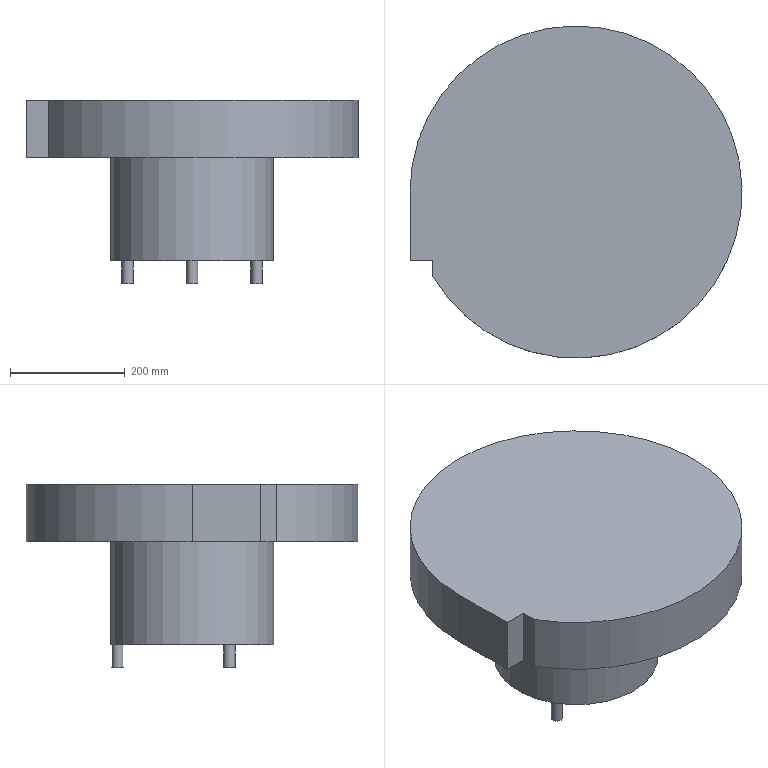Part | STEP file | ALIMENTADOR_PINO | 1 solid | 14 faces | box 580 x 580 x 320 mm | volume 38023743 mm3 | plane 9 | cylinder 5 | commonest cylinder face diameters 20 x3 285 x1 580 x1
STEP:
#1=CARTESIAN_POINT('',(0.,0.,0.));
#2=DIRECTION('',(0.,0.,1.));
#3=DIRECTION('',(1.,0.,0.));
#4=AXIS2_PLACEMENT_3D('',#1,#2,#3);
#5=CARTESIAN_POINT('',(-125.056,-68.318,40.));
#6=VERTEX_POINT('',#5);
#7=CARTESIAN_POINT('',(0.,0.,40.));
#8=DIRECTION('',(0.,0.,1.));
#9=DIRECTION('',(1.,0.,0.));
#10=AXIS2_PLACEMENT_3D('',#7,#8,#9);
#11=CIRCLE('',#10,142.5);
#12=CARTESIAN_POINT('',(-142.5,0.,40.));
#13=DIRECTION('',(0.,0.,1.));
#14=DIRECTION('',(1.,0.,0.));
#15=AXIS2_PLACEMENT_3D('',#12,#13,#14);
#16=PLANE('',#15);
#17=CARTESIAN_POINT('',(142.5,0.));
#18=DIRECTION('',(1.,0.));
#19=AXIS2_PLACEMENT_2D('',#17,#18);
#20=CIRCLE('',#19,142.5);
#21=(GEOMETRIC_REPRESENTATION_CONTEXT(2)PARAMETRIC_REPRESENTATION_CONTEXT()REPRESENTATION_CONTEXT('',''));
#22=DEFINITIONAL_REPRESENTATION('',(#20),#21);
#23=PCURVE('',#16,#22);
#24=CARTESIAN_POINT('',(0.,0.,180.));
#25=DIRECTION('',(0.,0.,1.));
#26=DIRECTION('',(-0.8776,-0.4794,0.));
#27=AXIS2_PLACEMENT_3D('',#24,#25,#26);
#28=CYLINDRICAL_SURFACE('',#27,142.5);
#29=CARTESIAN_POINT('',(-3.642,-140.));
#30=DIRECTION('',(1.,0.));
#31=VECTOR('',#30,1.);
#32=LINE('',#29,#31);
#33=(GEOMETRIC_REPRESENTATION_CONTEXT(2)PARAMETRIC_REPRESENTATION_CONTEXT()REPRESENTATION_CONTEXT('',''));
#34=DEFINITIONAL_REPRESENTATION('',(#32),#33);
#35=PCURVE('',#28,#34);
#36=SURFACE_CURVE('',#11,(#23,#35),.PCURVE_S1.);
#37=EDGE_CURVE('',#6,#6,#36,.T.);
#38=ORIENTED_EDGE('',*,*,#37,.F.);
#39=EDGE_LOOP('',(#38));
#40=FACE_BOUND('',#39,.T.);
#41=CARTESIAN_POINT('',(10.,130.,40.));
#42=VERTEX_POINT('',#41);
#43=CARTESIAN_POINT('',(0.,130.,40.));
#44=DIRECTION('',(0.,0.,1.));
#45=DIRECTION('',(1.,0.,0.));
#46=AXIS2_PLACEMENT_3D('',#43,#44,#45);
#47=CIRCLE('',#46,10.);
#48=CARTESIAN_POINT('',(142.5,130.));
#49=DIRECTION('',(1.,0.));
#50=AXIS2_PLACEMENT_2D('',#48,#49);
#51=CIRCLE('',#50,10.);
#52=(GEOMETRIC_REPRESENTATION_CONTEXT(2)PARAMETRIC_REPRESENTATION_CONTEXT()REPRESENTATION_CONTEXT('',''));
#53=DEFINITIONAL_REPRESENTATION('',(#51),#52);
#54=PCURVE('',#16,#53);
#55=CARTESIAN_POINT('',(0.,130.,20.));
#56=DIRECTION('',(0.,0.,-1.));
#57=DIRECTION('',(1.,0.,0.));
#58=AXIS2_PLACEMENT_3D('',#55,#56,#57);
#59=CYLINDRICAL_SURFACE('',#58,10.);
#60=CARTESIAN_POINT('',(6.283,-20.));
#61=DIRECTION('',(-1.,0.));
#62=VECTOR('',#61,1.);
#63=LINE('',#60,#62);
#64=(GEOMETRIC_REPRESENTATION_CONTEXT(2)PARAMETRIC_REPRESENTATION_CONTEXT()REPRESENTATION_CONTEXT('',''));
#65=DEFINITIONAL_REPRESENTATION('',(#63),#64);
#66=PCURVE('',#59,#65);
#67=SURFACE_CURVE('',#47,(#54,#66),.PCURVE_S1.);
#68=EDGE_CURVE('',#42,#42,#67,.T.);
#69=ORIENTED_EDGE('',*,*,#68,.T.);
#70=EDGE_LOOP('',(#69));
#71=FACE_BOUND('',#70,.T.);
#72=CARTESIAN_POINT('',(117.583,-56.34,40.));
#73=VERTEX_POINT('',#72);
#74=CARTESIAN_POINT('',(112.583,-65.,40.));
#75=DIRECTION('',(0.,0.,1.));
#76=DIRECTION('',(1.,0.,0.));
#77=AXIS2_PLACEMENT_3D('',#74,#75,#76);
#78=CIRCLE('',#77,10.);
#79=CARTESIAN_POINT('',(255.083,-65.));
#80=DIRECTION('',(1.,0.));
#81=AXIS2_PLACEMENT_2D('',#79,#80);
#82=CIRCLE('',#81,10.);
#83=(GEOMETRIC_REPRESENTATION_CONTEXT(2)PARAMETRIC_REPRESENTATION_CONTEXT()REPRESENTATION_CONTEXT('',''));
#84=DEFINITIONAL_REPRESENTATION('',(#82),#83);
#85=PCURVE('',#16,#84);
#86=CARTESIAN_POINT('',(112.583,-65.,20.));
#87=DIRECTION('',(0.,0.,-1.));
#88=DIRECTION('',(-0.5,-0.866,0.));
#89=AXIS2_PLACEMENT_3D('',#86,#87,#88);
#90=CYLINDRICAL_SURFACE('',#89,10.);
#91=CARTESIAN_POINT('',(10.472,-20.));
#92=DIRECTION('',(-1.,0.));
#93=VECTOR('',#92,1.);
#94=LINE('',#91,#93);
#95=(GEOMETRIC_REPRESENTATION_CONTEXT(2)PARAMETRIC_REPRESENTATION_CONTEXT()REPRESENTATION_CONTEXT('',''));
#96=DEFINITIONAL_REPRESENTATION('',(#94),#95);
#97=PCURVE('',#90,#96);
#98=SURFACE_CURVE('',#78,(#85,#97),.PCURVE_S1.);
#99=EDGE_CURVE('',#73,#73,#98,.T.);
#100=ORIENTED_EDGE('',*,*,#99,.T.);
#101=EDGE_LOOP('',(#100));
#102=FACE_BOUND('',#101,.T.);
#103=CARTESIAN_POINT('',(-107.583,-73.66,40.));
#104=VERTEX_POINT('',#103);
#105=CARTESIAN_POINT('',(-112.583,-65.,40.));
#106=DIRECTION('',(0.,0.,1.));
#107=DIRECTION('',(1.,0.,0.));
#108=AXIS2_PLACEMENT_3D('',#105,#106,#107);
#109=CIRCLE('',#108,10.);
#110=CARTESIAN_POINT('',(29.917,-65.));
#111=DIRECTION('',(1.,0.));
#112=AXIS2_PLACEMENT_2D('',#110,#111);
#113=CIRCLE('',#112,10.);
#114=(GEOMETRIC_REPRESENTATION_CONTEXT(2)PARAMETRIC_REPRESENTATION_CONTEXT()REPRESENTATION_CONTEXT('',''));
#115=DEFINITIONAL_REPRESENTATION('',(#113),#114);
#116=PCURVE('',#16,#115);
#117=CARTESIAN_POINT('',(-112.583,-65.,20.));
#118=DIRECTION('',(0.,0.,-1.));
#119=DIRECTION('',(-0.5,0.866,0.));
#120=AXIS2_PLACEMENT_3D('',#117,#118,#119);
#121=CYLINDRICAL_SURFACE('',#120,10.);
#122=CARTESIAN_POINT('',(14.661,-20.));
#123=DIRECTION('',(-1.,0.));
#124=VECTOR('',#123,1.);
#125=LINE('',#122,#124);
#126=(GEOMETRIC_REPRESENTATION_CONTEXT(2)PARAMETRIC_REPRESENTATION_CONTEXT()REPRESENTATION_CONTEXT('',''));
#127=DEFINITIONAL_REPRESENTATION('',(#125),#126);
#128=PCURVE('',#121,#127);
#129=SURFACE_CURVE('',#109,(#116,#128),.PCURVE_S1.);
#130=EDGE_CURVE('',#104,#104,#129,.T.);
#131=ORIENTED_EDGE('',*,*,#130,.T.);
#132=EDGE_LOOP('',(#131));
#133=FACE_BOUND('',#132,.T.);
#134=ADVANCED_FACE('',(#40,#71,#102,#133),#16,.F.);
#135=CARTESIAN_POINT('',(-250.,-146.969,220.));
#136=VERTEX_POINT('',#135);
#137=CARTESIAN_POINT('',(-290.,0.,220.));
#138=VERTEX_POINT('',#137);
#139=CARTESIAN_POINT('',(0.,0.,220.));
#140=DIRECTION('',(0.,0.,1.));
#141=DIRECTION('',(1.,0.,0.));
#142=AXIS2_PLACEMENT_3D('',#139,#140,#141);
#143=CIRCLE('',#142,290.);
#144=CARTESIAN_POINT('',(0.,0.,180.));
#145=DIRECTION('',(0.,0.,1.));
#146=DIRECTION('',(-0.8776,-0.4794,0.));
#147=AXIS2_PLACEMENT_3D('',#144,#145,#146);
#148=CYLINDRICAL_SURFACE('',#147,290.);
#149=CARTESIAN_POINT('',(-3.642,40.));
#150=DIRECTION('',(1.,0.));
#151=VECTOR('',#150,1.);
#152=LINE('',#149,#151);
#153=(GEOMETRIC_REPRESENTATION_CONTEXT(2)PARAMETRIC_REPRESENTATION_CONTEXT()REPRESENTATION_CONTEXT('',''));
#154=DEFINITIONAL_REPRESENTATION('',(#152),#153);
#155=PCURVE('',#148,#154);
#156=CARTESIAN_POINT('',(-142.5,0.,220.));
#157=DIRECTION('',(0.,0.,1.));
#158=DIRECTION('',(1.,0.,0.));
#159=AXIS2_PLACEMENT_3D('',#156,#157,#158);
#160=PLANE('',#159);
#161=CARTESIAN_POINT('',(142.5,0.));
#162=DIRECTION('',(1.,0.));
#163=AXIS2_PLACEMENT_2D('',#161,#162);
#164=CIRCLE('',#163,290.);
#165=(GEOMETRIC_REPRESENTATION_CONTEXT(2)PARAMETRIC_REPRESENTATION_CONTEXT()REPRESENTATION_CONTEXT('',''));
#166=DEFINITIONAL_REPRESENTATION('',(#164),#165);
#167=PCURVE('',#160,#166);
#168=SURFACE_CURVE('',#143,(#155,#167),.PCURVE_S1.);
#169=EDGE_CURVE('',#136,#138,#168,.T.);
#170=ORIENTED_EDGE('',*,*,#169,.T.);
#171=CARTESIAN_POINT('',(-290.,0.,320.));
#172=VERTEX_POINT('',#171);
#173=CARTESIAN_POINT('',(-290.,0.,220.));
#174=DIRECTION('',(0.,0.,1.));
#175=VECTOR('',#174,1.);
#176=LINE('',#173,#175);
#177=CARTESIAN_POINT('',(5.783,40.));
#178=DIRECTION('',(0.,1.));
#179=VECTOR('',#178,1.);
#180=LINE('',#177,#179);
#181=(GEOMETRIC_REPRESENTATION_CONTEXT(2)PARAMETRIC_REPRESENTATION_CONTEXT()REPRESENTATION_CONTEXT('',''));
#182=DEFINITIONAL_REPRESENTATION('',(#180),#181);
#183=PCURVE('',#148,#182);
#184=CARTESIAN_POINT('',(-290.,0.,320.));
#185=DIRECTION('',(1.,0.,0.));
#186=DIRECTION('',(0.,0.,-1.));
#187=AXIS2_PLACEMENT_3D('',#184,#185,#186);
#188=PLANE('',#187);
#189=CARTESIAN_POINT('',(100.,0.));
#190=DIRECTION('',(-1.,0.));
#191=VECTOR('',#190,1.);
#192=LINE('',#189,#191);
#193=(GEOMETRIC_REPRESENTATION_CONTEXT(2)PARAMETRIC_REPRESENTATION_CONTEXT()REPRESENTATION_CONTEXT('',''));
#194=DEFINITIONAL_REPRESENTATION('',(#192),#193);
#195=PCURVE('',#188,#194);
#196=SURFACE_CURVE('',#176,(#183,#195),.PCURVE_S1.);
#197=EDGE_CURVE('',#138,#172,#196,.T.);
#198=ORIENTED_EDGE('',*,*,#197,.T.);
#199=CARTESIAN_POINT('',(-250.,-146.969,320.));
#200=VERTEX_POINT('',#199);
#201=CARTESIAN_POINT('',(0.,0.,320.));
#202=DIRECTION('',(0.,0.,1.));
#203=DIRECTION('',(1.,0.,0.));
#204=AXIS2_PLACEMENT_3D('',#201,#202,#203);
#205=CIRCLE('',#204,290.);
#206=CARTESIAN_POINT('',(-3.642,140.));
#207=DIRECTION('',(1.,0.));
#208=VECTOR('',#207,1.);
#209=LINE('',#206,#208);
#210=(GEOMETRIC_REPRESENTATION_CONTEXT(2)PARAMETRIC_REPRESENTATION_CONTEXT()REPRESENTATION_CONTEXT('',''));
#211=DEFINITIONAL_REPRESENTATION('',(#209),#210);
#212=PCURVE('',#148,#211);
#213=CARTESIAN_POINT('',(-290.,0.,320.));
#214=DIRECTION('',(0.,0.,1.));
#215=DIRECTION('',(1.,0.,0.));
#216=AXIS2_PLACEMENT_3D('',#213,#214,#215);
#217=PLANE('',#216);
#218=CARTESIAN_POINT('',(290.,0.));
#219=DIRECTION('',(1.,0.));
#220=AXIS2_PLACEMENT_2D('',#218,#219);
#221=CIRCLE('',#220,290.);
#222=(GEOMETRIC_REPRESENTATION_CONTEXT(2)PARAMETRIC_REPRESENTATION_CONTEXT()REPRESENTATION_CONTEXT('',''));
#223=DEFINITIONAL_REPRESENTATION('',(#221),#222);
#224=PCURVE('',#217,#223);
#225=SURFACE_CURVE('',#205,(#212,#224),.PCURVE_S1.);
#226=EDGE_CURVE('',#200,#172,#225,.T.);
#227=ORIENTED_EDGE('',*,*,#226,.F.);
#228=CARTESIAN_POINT('',(-250.,-146.969,220.));
#229=DIRECTION('',(0.,0.,1.));
#230=VECTOR('',#229,1.);
#231=LINE('',#228,#230);
#232=CARTESIAN_POINT('',(0.03146,40.));
#233=DIRECTION('',(0.,1.));
#234=VECTOR('',#233,1.);
#235=LINE('',#232,#234);
#236=(GEOMETRIC_REPRESENTATION_CONTEXT(2)PARAMETRIC_REPRESENTATION_CONTEXT()REPRESENTATION_CONTEXT('',''));
#237=DEFINITIONAL_REPRESENTATION('',(#235),#236);
#238=PCURVE('',#148,#237);
#239=CARTESIAN_POINT('',(-250.,-120.,320.));
#240=DIRECTION('',(1.,0.,0.));
#241=DIRECTION('',(0.,0.,-1.));
#242=AXIS2_PLACEMENT_3D('',#239,#240,#241);
#243=PLANE('',#242);
#244=CARTESIAN_POINT('',(100.,-26.969));
#245=DIRECTION('',(-1.,0.));
#246=VECTOR('',#245,1.);
#247=LINE('',#244,#246);
#248=(GEOMETRIC_REPRESENTATION_CONTEXT(2)PARAMETRIC_REPRESENTATION_CONTEXT()REPRESENTATION_CONTEXT('',''));
#249=DEFINITIONAL_REPRESENTATION('',(#247),#248);
#250=PCURVE('',#243,#249);
#251=SURFACE_CURVE('',#231,(#238,#250),.PCURVE_S1.);
#252=EDGE_CURVE('',#136,#200,#251,.T.);
#253=ORIENTED_EDGE('',*,*,#252,.F.);
#254=EDGE_LOOP('',(#170,#198,#227,#253));
#255=FACE_BOUND('',#254,.T.);
#256=ADVANCED_FACE('',(#255),#148,.T.);
#257=ORIENTED_EDGE('',*,*,#37,.T.);
#258=CARTESIAN_POINT('',(-125.056,-68.318,220.));
#259=VERTEX_POINT('',#258);
#260=CARTESIAN_POINT('',(-125.056,-68.318,40.));
#261=CARTESIAN_POINT('',(-125.056,-68.318,220.));
#262=B_SPLINE_CURVE_WITH_KNOTS('',1,(#260,#261),.UNSPECIFIED.,.F.,.F.,(2,2),(-140.,40.),.PIECEWISE_BEZIER_KNOTS.);
#263=CARTESIAN_POINT('',(6.283,0.));
#264=DIRECTION('',(0.,1.));
#265=VECTOR('',#264,1.);
#266=LINE('',#263,#265);
#267=(GEOMETRIC_REPRESENTATION_CONTEXT(2)PARAMETRIC_REPRESENTATION_CONTEXT()REPRESENTATION_CONTEXT('',''));
#268=DEFINITIONAL_REPRESENTATION('',(#266),#267);
#269=PCURVE('',#28,#268);
#270=CARTESIAN_POINT('',(0.,0.));
#271=DIRECTION('',(0.,1.));
#272=VECTOR('',#271,1.);
#273=LINE('',#270,#272);
#274=(GEOMETRIC_REPRESENTATION_CONTEXT(2)PARAMETRIC_REPRESENTATION_CONTEXT()REPRESENTATION_CONTEXT('',''));
#275=DEFINITIONAL_REPRESENTATION('',(#273),#274);
#276=PCURVE('',#28,#275);
#277=SEAM_CURVE('',#262,(#269,#276),.PCURVE_S1.);
#278=EDGE_CURVE('',#6,#259,#277,.T.);
#279=ORIENTED_EDGE('',*,*,#278,.T.);
#280=CARTESIAN_POINT('',(0.,0.,220.));
#281=DIRECTION('',(0.,0.,1.));
#282=DIRECTION('',(1.,0.,0.));
#283=AXIS2_PLACEMENT_3D('',#280,#281,#282);
#284=CIRCLE('',#283,142.5);
#285=CARTESIAN_POINT('',(-3.642,40.));
#286=DIRECTION('',(1.,0.));
#287=VECTOR('',#286,1.);
#288=LINE('',#285,#287);
#289=(GEOMETRIC_REPRESENTATION_CONTEXT(2)PARAMETRIC_REPRESENTATION_CONTEXT()REPRESENTATION_CONTEXT('',''));
#290=DEFINITIONAL_REPRESENTATION('',(#288),#289);
#291=PCURVE('',#28,#290);
#292=CARTESIAN_POINT('',(142.5,0.));
#293=DIRECTION('',(1.,0.));
#294=AXIS2_PLACEMENT_2D('',#292,#293);
#295=CIRCLE('',#294,142.5);
#296=(GEOMETRIC_REPRESENTATION_CONTEXT(2)PARAMETRIC_REPRESENTATION_CONTEXT()REPRESENTATION_CONTEXT('',''));
#297=DEFINITIONAL_REPRESENTATION('',(#295),#296);
#298=PCURVE('',#160,#297);
#299=SURFACE_CURVE('',#284,(#291,#298),.PCURVE_S1.);
#300=EDGE_CURVE('',#259,#259,#299,.T.);
#301=ORIENTED_EDGE('',*,*,#300,.F.);
#302=ORIENTED_EDGE('',*,*,#278,.F.);
#303=EDGE_LOOP('',(#257,#279,#301,#302));
#304=FACE_BOUND('',#303,.T.);
#305=ADVANCED_FACE('',(#304),#28,.T.);
#306=CARTESIAN_POINT('',(-290.,-120.,220.));
#307=VERTEX_POINT('',#306);
#308=CARTESIAN_POINT('',(-290.,0.,220.));
#309=DIRECTION('',(0.,-1.,0.));
#310=VECTOR('',#309,1.);
#311=LINE('',#308,#310);
#312=CARTESIAN_POINT('',(100.,0.));
#313=DIRECTION('',(0.,-1.));
#314=VECTOR('',#313,1.);
#315=LINE('',#312,#314);
#316=(GEOMETRIC_REPRESENTATION_CONTEXT(2)PARAMETRIC_REPRESENTATION_CONTEXT()REPRESENTATION_CONTEXT('',''));
#317=DEFINITIONAL_REPRESENTATION('',(#315),#316);
#318=PCURVE('',#188,#317);
#319=CARTESIAN_POINT('',(-147.5,0.));
#320=DIRECTION('',(0.,-1.));
#321=VECTOR('',#320,1.);
#322=LINE('',#319,#321);
#323=(GEOMETRIC_REPRESENTATION_CONTEXT(2)PARAMETRIC_REPRESENTATION_CONTEXT()REPRESENTATION_CONTEXT('',''));
#324=DEFINITIONAL_REPRESENTATION('',(#322),#323);
#325=PCURVE('',#160,#324);
#326=SURFACE_CURVE('',#311,(#318,#325),.PCURVE_S1.);
#327=EDGE_CURVE('',#138,#307,#326,.T.);
#328=ORIENTED_EDGE('',*,*,#327,.T.);
#329=CARTESIAN_POINT('',(-290.,-120.,320.));
#330=VERTEX_POINT('',#329);
#331=CARTESIAN_POINT('',(-290.,-120.,320.));
#332=DIRECTION('',(0.,0.,-1.));
#333=VECTOR('',#332,1.);
#334=LINE('',#331,#333);
#335=CARTESIAN_POINT('',(0.,-120.));
#336=DIRECTION('',(1.,0.));
#337=VECTOR('',#336,1.);
#338=LINE('',#335,#337);
#339=(GEOMETRIC_REPRESENTATION_CONTEXT(2)PARAMETRIC_REPRESENTATION_CONTEXT()REPRESENTATION_CONTEXT('',''));
#340=DEFINITIONAL_REPRESENTATION('',(#338),#339);
#341=PCURVE('',#188,#340);
#342=CARTESIAN_POINT('',(-250.,-120.,320.));
#343=DIRECTION('',(0.,-1.,0.));
#344=DIRECTION('',(0.,0.,-1.));
#345=AXIS2_PLACEMENT_3D('',#342,#343,#344);
#346=PLANE('',#345);
#347=CARTESIAN_POINT('',(0.,-40.));
#348=DIRECTION('',(1.,0.));
#349=VECTOR('',#348,1.);
#350=LINE('',#347,#349);
#351=(GEOMETRIC_REPRESENTATION_CONTEXT(2)PARAMETRIC_REPRESENTATION_CONTEXT()REPRESENTATION_CONTEXT('',''));
#352=DEFINITIONAL_REPRESENTATION('',(#350),#351);
#353=PCURVE('',#346,#352);
#354=SURFACE_CURVE('',#334,(#341,#353),.PCURVE_S1.);
#355=EDGE_CURVE('',#330,#307,#354,.T.);
#356=ORIENTED_EDGE('',*,*,#355,.F.);
#357=CARTESIAN_POINT('',(-290.,0.,320.));
#358=DIRECTION('',(0.,-1.,0.));
#359=VECTOR('',#358,1.);
#360=LINE('',#357,#359);
#361=CARTESIAN_POINT('',(0.,0.));
#362=DIRECTION('',(0.,-1.));
#363=VECTOR('',#362,1.);
#364=LINE('',#361,#363);
#365=(GEOMETRIC_REPRESENTATION_CONTEXT(2)PARAMETRIC_REPRESENTATION_CONTEXT()REPRESENTATION_CONTEXT('',''));
#366=DEFINITIONAL_REPRESENTATION('',(#364),#365);
#367=PCURVE('',#188,#366);
#368=CARTESIAN_POINT('',(0.,0.));
#369=DIRECTION('',(0.,-1.));
#370=VECTOR('',#369,1.);
#371=LINE('',#368,#370);
#372=(GEOMETRIC_REPRESENTATION_CONTEXT(2)PARAMETRIC_REPRESENTATION_CONTEXT()REPRESENTATION_CONTEXT('',''));
#373=DEFINITIONAL_REPRESENTATION('',(#371),#372);
#374=PCURVE('',#217,#373);
#375=SURFACE_CURVE('',#360,(#367,#374),.PCURVE_S1.);
#376=EDGE_CURVE('',#172,#330,#375,.T.);
#377=ORIENTED_EDGE('',*,*,#376,.F.);
#378=ORIENTED_EDGE('',*,*,#197,.F.);
#379=EDGE_LOOP('',(#328,#356,#377,#378));
#380=FACE_BOUND('',#379,.T.);
#381=ADVANCED_FACE('',(#380),#188,.F.);
#382=CARTESIAN_POINT('',(-250.,-120.,320.));
#383=VERTEX_POINT('',#382);
#384=CARTESIAN_POINT('',(-250.,-120.,220.));
#385=VERTEX_POINT('',#384);
#386=CARTESIAN_POINT('',(-250.,-120.,320.));
#387=DIRECTION('',(0.,0.,-1.));
#388=VECTOR('',#387,1.);
#389=LINE('',#386,#388);
#390=CARTESIAN_POINT('',(0.,0.));
#391=DIRECTION('',(1.,0.));
#392=VECTOR('',#391,1.);
#393=LINE('',#390,#392);
#394=(GEOMETRIC_REPRESENTATION_CONTEXT(2)PARAMETRIC_REPRESENTATION_CONTEXT()REPRESENTATION_CONTEXT('',''));
#395=DEFINITIONAL_REPRESENTATION('',(#393),#394);
#396=PCURVE('',#346,#395);
#397=CARTESIAN_POINT('',(0.,0.));
#398=DIRECTION('',(1.,0.));
#399=VECTOR('',#398,1.);
#400=LINE('',#397,#399);
#401=(GEOMETRIC_REPRESENTATION_CONTEXT(2)PARAMETRIC_REPRESENTATION_CONTEXT()REPRESENTATION_CONTEXT('',''));
#402=DEFINITIONAL_REPRESENTATION('',(#400),#401);
#403=PCURVE('',#243,#402);
#404=SURFACE_CURVE('',#389,(#396,#403),.PCURVE_S1.);
#405=EDGE_CURVE('',#383,#385,#404,.T.);
#406=ORIENTED_EDGE('',*,*,#405,.F.);
#407=CARTESIAN_POINT('',(-290.,-120.,320.));
#408=DIRECTION('',(1.,0.,0.));
#409=VECTOR('',#408,1.);
#410=LINE('',#407,#409);
#411=CARTESIAN_POINT('',(0.,-40.));
#412=DIRECTION('',(0.,1.));
#413=VECTOR('',#412,1.);
#414=LINE('',#411,#413);
#415=(GEOMETRIC_REPRESENTATION_CONTEXT(2)PARAMETRIC_REPRESENTATION_CONTEXT()REPRESENTATION_CONTEXT('',''));
#416=DEFINITIONAL_REPRESENTATION('',(#414),#415);
#417=PCURVE('',#346,#416);
#418=CARTESIAN_POINT('',(0.,-120.));
#419=DIRECTION('',(1.,0.));
#420=VECTOR('',#419,1.);
#421=LINE('',#418,#420);
#422=(GEOMETRIC_REPRESENTATION_CONTEXT(2)PARAMETRIC_REPRESENTATION_CONTEXT()REPRESENTATION_CONTEXT('',''));
#423=DEFINITIONAL_REPRESENTATION('',(#421),#422);
#424=PCURVE('',#217,#423);
#425=SURFACE_CURVE('',#410,(#417,#424),.PCURVE_S1.);
#426=EDGE_CURVE('',#330,#383,#425,.T.);
#427=ORIENTED_EDGE('',*,*,#426,.F.);
#428=ORIENTED_EDGE('',*,*,#355,.T.);
#429=CARTESIAN_POINT('',(-250.,-120.,220.));
#430=DIRECTION('',(-1.,0.,0.));
#431=VECTOR('',#430,1.);
#432=LINE('',#429,#431);
#433=CARTESIAN_POINT('',(100.,0.));
#434=DIRECTION('',(0.,-1.));
#435=VECTOR('',#434,1.);
#436=LINE('',#433,#435);
#437=(GEOMETRIC_REPRESENTATION_CONTEXT(2)PARAMETRIC_REPRESENTATION_CONTEXT()REPRESENTATION_CONTEXT('',''));
#438=DEFINITIONAL_REPRESENTATION('',(#436),#437);
#439=PCURVE('',#346,#438);
#440=CARTESIAN_POINT('',(-107.5,-120.));
#441=DIRECTION('',(-1.,0.));
#442=VECTOR('',#441,1.);
#443=LINE('',#440,#442);
#444=(GEOMETRIC_REPRESENTATION_CONTEXT(2)PARAMETRIC_REPRESENTATION_CONTEXT()REPRESENTATION_CONTEXT('',''));
#445=DEFINITIONAL_REPRESENTATION('',(#443),#444);
#446=PCURVE('',#160,#445);
#447=SURFACE_CURVE('',#432,(#439,#446),.PCURVE_S1.);
#448=EDGE_CURVE('',#385,#307,#447,.T.);
#449=ORIENTED_EDGE('',*,*,#448,.F.);
#450=EDGE_LOOP('',(#406,#427,#428,#449));
#451=FACE_BOUND('',#450,.T.);
#452=ADVANCED_FACE('',(#451),#346,.T.);
#453=CARTESIAN_POINT('',(-250.,-120.,220.));
#454=DIRECTION('',(0.,-1.,0.));
#455=VECTOR('',#454,1.);
#456=LINE('',#453,#455);
#457=CARTESIAN_POINT('',(-107.5,-120.));
#458=DIRECTION('',(0.,-1.));
#459=VECTOR('',#458,1.);
#460=LINE('',#457,#459);
#461=(GEOMETRIC_REPRESENTATION_CONTEXT(2)PARAMETRIC_REPRESENTATION_CONTEXT()REPRESENTATION_CONTEXT('',''));
#462=DEFINITIONAL_REPRESENTATION('',(#460),#461);
#463=PCURVE('',#160,#462);
#464=CARTESIAN_POINT('',(100.,0.));
#465=DIRECTION('',(0.,-1.));
#466=VECTOR('',#465,1.);
#467=LINE('',#464,#466);
#468=(GEOMETRIC_REPRESENTATION_CONTEXT(2)PARAMETRIC_REPRESENTATION_CONTEXT()REPRESENTATION_CONTEXT('',''));
#469=DEFINITIONAL_REPRESENTATION('',(#467),#468);
#470=PCURVE('',#243,#469);
#471=SURFACE_CURVE('',#456,(#463,#470),.PCURVE_S1.);
#472=EDGE_CURVE('',#385,#136,#471,.T.);
#473=ORIENTED_EDGE('',*,*,#472,.F.);
#474=ORIENTED_EDGE('',*,*,#448,.T.);
#475=ORIENTED_EDGE('',*,*,#327,.F.);
#476=ORIENTED_EDGE('',*,*,#169,.F.);
#477=EDGE_LOOP('',(#473,#474,#475,#476));
#478=FACE_BOUND('',#477,.T.);
#479=ORIENTED_EDGE('',*,*,#300,.T.);
#480=EDGE_LOOP('',(#479));
#481=FACE_BOUND('',#480,.T.);
#482=ADVANCED_FACE('',(#478,#481),#160,.F.);
#483=ORIENTED_EDGE('',*,*,#226,.T.);
#484=ORIENTED_EDGE('',*,*,#376,.T.);
#485=ORIENTED_EDGE('',*,*,#426,.T.);
#486=CARTESIAN_POINT('',(-250.,-120.,320.));
#487=DIRECTION('',(0.,-1.,0.));
#488=VECTOR('',#487,1.);
#489=LINE('',#486,#488);
#490=CARTESIAN_POINT('',(40.,-120.));
#491=DIRECTION('',(0.,-1.));
#492=VECTOR('',#491,1.);
#493=LINE('',#490,#492);
#494=(GEOMETRIC_REPRESENTATION_CONTEXT(2)PARAMETRIC_REPRESENTATION_CONTEXT()REPRESENTATION_CONTEXT('',''));
#495=DEFINITIONAL_REPRESENTATION('',(#493),#494);
#496=PCURVE('',#217,#495);
#497=CARTESIAN_POINT('',(0.,0.));
#498=DIRECTION('',(0.,-1.));
#499=VECTOR('',#498,1.);
#500=LINE('',#497,#499);
#501=(GEOMETRIC_REPRESENTATION_CONTEXT(2)PARAMETRIC_REPRESENTATION_CONTEXT()REPRESENTATION_CONTEXT('',''));
#502=DEFINITIONAL_REPRESENTATION('',(#500),#501);
#503=PCURVE('',#243,#502);
#504=SURFACE_CURVE('',#489,(#496,#503),.PCURVE_S1.);
#505=EDGE_CURVE('',#383,#200,#504,.T.);
#506=ORIENTED_EDGE('',*,*,#505,.T.);
#507=EDGE_LOOP('',(#483,#484,#485,#506));
#508=FACE_BOUND('',#507,.T.);
#509=ADVANCED_FACE('',(#508),#217,.T.);
#510=ORIENTED_EDGE('',*,*,#472,.T.);
#511=ORIENTED_EDGE('',*,*,#252,.T.);
#512=ORIENTED_EDGE('',*,*,#505,.F.);
#513=ORIENTED_EDGE('',*,*,#405,.T.);
#514=EDGE_LOOP('',(#510,#511,#512,#513));
#515=FACE_BOUND('',#514,.T.);
#516=ADVANCED_FACE('',(#515),#243,.F.);
#517=CARTESIAN_POINT('',(10.,130.,0.));
#518=VERTEX_POINT('',#517);
#519=CARTESIAN_POINT('',(0.,130.,0.));
#520=DIRECTION('',(0.,0.,-1.));
#521=DIRECTION('',(1.,0.,0.));
#522=AXIS2_PLACEMENT_3D('',#519,#520,#521);
#523=CIRCLE('',#522,10.);
#524=CARTESIAN_POINT('',(0.,0.,0.));
#525=DIRECTION('',(0.,0.,-1.));
#526=DIRECTION('',(-1.,0.,0.));
#527=AXIS2_PLACEMENT_3D('',#524,#525,#526);
#528=PLANE('',#527);
#529=CARTESIAN_POINT('',(0.,130.));
#530=DIRECTION('',(-1.,0.));
#531=AXIS2_PLACEMENT_2D('',#529,#530);
#532=CIRCLE('',#531,10.);
#533=(GEOMETRIC_REPRESENTATION_CONTEXT(2)PARAMETRIC_REPRESENTATION_CONTEXT()REPRESENTATION_CONTEXT('',''));
#534=DEFINITIONAL_REPRESENTATION('',(#532),#533);
#535=PCURVE('',#528,#534);
#536=CARTESIAN_POINT('',(0.,20.));
#537=DIRECTION('',(1.,0.));
#538=VECTOR('',#537,1.);
#539=LINE('',#536,#538);
#540=(GEOMETRIC_REPRESENTATION_CONTEXT(2)PARAMETRIC_REPRESENTATION_CONTEXT()REPRESENTATION_CONTEXT('',''));
#541=DEFINITIONAL_REPRESENTATION('',(#539),#540);
#542=PCURVE('',#59,#541);
#543=SURFACE_CURVE('',#523,(#535,#542),.PCURVE_S1.);
#544=EDGE_CURVE('',#518,#518,#543,.T.);
#545=ORIENTED_EDGE('',*,*,#544,.T.);
#546=EDGE_LOOP('',(#545));
#547=FACE_BOUND('',#546,.T.);
#548=ADVANCED_FACE('',(#547),#528,.T.);
#549=ORIENTED_EDGE('',*,*,#544,.F.);
#550=CARTESIAN_POINT('',(10.,130.,40.));
#551=CARTESIAN_POINT('',(10.,130.,0.));
#552=B_SPLINE_CURVE_WITH_KNOTS('',1,(#550,#551),.UNSPECIFIED.,.F.,.F.,(2,2),(-20.,20.),.PIECEWISE_BEZIER_KNOTS.);
#553=CARTESIAN_POINT('',(0.,0.));
#554=DIRECTION('',(0.,1.));
#555=VECTOR('',#554,1.);
#556=LINE('',#553,#555);
#557=(GEOMETRIC_REPRESENTATION_CONTEXT(2)PARAMETRIC_REPRESENTATION_CONTEXT()REPRESENTATION_CONTEXT('',''));
#558=DEFINITIONAL_REPRESENTATION('',(#556),#557);
#559=PCURVE('',#59,#558);
#560=CARTESIAN_POINT('',(6.283,0.));
#561=DIRECTION('',(0.,1.));
#562=VECTOR('',#561,1.);
#563=LINE('',#560,#562);
#564=(GEOMETRIC_REPRESENTATION_CONTEXT(2)PARAMETRIC_REPRESENTATION_CONTEXT()REPRESENTATION_CONTEXT('',''));
#565=DEFINITIONAL_REPRESENTATION('',(#563),#564);
#566=PCURVE('',#59,#565);
#567=SEAM_CURVE('',#552,(#559,#566),.PCURVE_S1.);
#568=EDGE_CURVE('',#42,#518,#567,.T.);
#569=ORIENTED_EDGE('',*,*,#568,.F.);
#570=ORIENTED_EDGE('',*,*,#68,.F.);
#571=ORIENTED_EDGE('',*,*,#568,.T.);
#572=EDGE_LOOP('',(#549,#569,#570,#571));
#573=FACE_BOUND('',#572,.T.);
#574=ADVANCED_FACE('',(#573),#59,.T.);
#575=CARTESIAN_POINT('',(-107.583,-73.66,0.));
#576=VERTEX_POINT('',#575);
#577=CARTESIAN_POINT('',(-112.583,-65.,0.));
#578=DIRECTION('',(0.,0.,-1.));
#579=DIRECTION('',(1.,0.,0.));
#580=AXIS2_PLACEMENT_3D('',#577,#578,#579);
#581=CIRCLE('',#580,10.);
#582=CARTESIAN_POINT('',(2.094,20.));
#583=DIRECTION('',(1.,0.));
#584=VECTOR('',#583,1.);
#585=LINE('',#582,#584);
#586=(GEOMETRIC_REPRESENTATION_CONTEXT(2)PARAMETRIC_REPRESENTATION_CONTEXT()REPRESENTATION_CONTEXT('',''));
#587=DEFINITIONAL_REPRESENTATION('',(#585),#586);
#588=PCURVE('',#121,#587);
#589=CARTESIAN_POINT('',(0.,0.,0.));
#590=DIRECTION('',(0.,0.,-1.));
#591=DIRECTION('',(-1.,0.,0.));
#592=AXIS2_PLACEMENT_3D('',#589,#590,#591);
#593=PLANE('',#592);
#594=CARTESIAN_POINT('',(112.583,-65.));
#595=DIRECTION('',(-1.,0.));
#596=AXIS2_PLACEMENT_2D('',#594,#595);
#597=CIRCLE('',#596,10.);
#598=(GEOMETRIC_REPRESENTATION_CONTEXT(2)PARAMETRIC_REPRESENTATION_CONTEXT()REPRESENTATION_CONTEXT('',''));
#599=DEFINITIONAL_REPRESENTATION('',(#597),#598);
#600=PCURVE('',#593,#599);
#601=SURFACE_CURVE('',#581,(#588,#600),.PCURVE_S1.);
#602=EDGE_CURVE('',#576,#576,#601,.T.);
#603=ORIENTED_EDGE('',*,*,#602,.F.);
#604=CARTESIAN_POINT('',(-107.583,-73.66,40.));
#605=CARTESIAN_POINT('',(-107.583,-73.66,0.));
#606=B_SPLINE_CURVE_WITH_KNOTS('',1,(#604,#605),.UNSPECIFIED.,.F.,.F.,(2,2),(-20.,20.),.PIECEWISE_BEZIER_KNOTS.);
#607=CARTESIAN_POINT('',(3.142,0.));
#608=DIRECTION('',(0.,1.));
#609=VECTOR('',#608,1.);
#610=LINE('',#607,#609);
#611=(GEOMETRIC_REPRESENTATION_CONTEXT(2)PARAMETRIC_REPRESENTATION_CONTEXT()REPRESENTATION_CONTEXT('',''));
#612=DEFINITIONAL_REPRESENTATION('',(#610),#611);
#613=PCURVE('',#121,#612);
#614=CARTESIAN_POINT('',(9.425,0.));
#615=DIRECTION('',(0.,1.));
#616=VECTOR('',#615,1.);
#617=LINE('',#614,#616);
#618=(GEOMETRIC_REPRESENTATION_CONTEXT(2)PARAMETRIC_REPRESENTATION_CONTEXT()REPRESENTATION_CONTEXT('',''));
#619=DEFINITIONAL_REPRESENTATION('',(#617),#618);
#620=PCURVE('',#121,#619);
#621=SEAM_CURVE('',#606,(#613,#620),.PCURVE_S1.);
#622=EDGE_CURVE('',#104,#576,#621,.T.);
#623=ORIENTED_EDGE('',*,*,#622,.F.);
#624=ORIENTED_EDGE('',*,*,#130,.F.);
#625=ORIENTED_EDGE('',*,*,#622,.T.);
#626=EDGE_LOOP('',(#603,#623,#624,#625));
#627=FACE_BOUND('',#626,.T.);
#628=ADVANCED_FACE('',(#627),#121,.T.);
#629=ORIENTED_EDGE('',*,*,#602,.T.);
#630=EDGE_LOOP('',(#629));
#631=FACE_BOUND('',#630,.T.);
#632=ADVANCED_FACE('',(#631),#593,.T.);
#633=CARTESIAN_POINT('',(117.583,-56.34,0.));
#634=VERTEX_POINT('',#633);
#635=CARTESIAN_POINT('',(112.583,-65.,0.));
#636=DIRECTION('',(0.,0.,-1.));
#637=DIRECTION('',(1.,0.,0.));
#638=AXIS2_PLACEMENT_3D('',#635,#636,#637);
#639=CIRCLE('',#638,10.);
#640=CARTESIAN_POINT('',(-2.094,20.));
#641=DIRECTION('',(1.,0.));
#642=VECTOR('',#641,1.);
#643=LINE('',#640,#642);
#644=(GEOMETRIC_REPRESENTATION_CONTEXT(2)PARAMETRIC_REPRESENTATION_CONTEXT()REPRESENTATION_CONTEXT('',''));
#645=DEFINITIONAL_REPRESENTATION('',(#643),#644);
#646=PCURVE('',#90,#645);
#647=CARTESIAN_POINT('',(0.,0.,0.));
#648=DIRECTION('',(0.,0.,-1.));
#649=DIRECTION('',(-1.,0.,0.));
#650=AXIS2_PLACEMENT_3D('',#647,#648,#649);
#651=PLANE('',#650);
#652=CARTESIAN_POINT('',(-112.583,-65.));
#653=DIRECTION('',(-1.,0.));
#654=AXIS2_PLACEMENT_2D('',#652,#653);
#655=CIRCLE('',#654,10.);
#656=(GEOMETRIC_REPRESENTATION_CONTEXT(2)PARAMETRIC_REPRESENTATION_CONTEXT()REPRESENTATION_CONTEXT('',''));
#657=DEFINITIONAL_REPRESENTATION('',(#655),#656);
#658=PCURVE('',#651,#657);
#659=SURFACE_CURVE('',#639,(#646,#658),.PCURVE_S1.);
#660=EDGE_CURVE('',#634,#634,#659,.T.);
#661=ORIENTED_EDGE('',*,*,#660,.F.);
#662=CARTESIAN_POINT('',(117.583,-56.34,40.));
#663=CARTESIAN_POINT('',(117.583,-56.34,0.));
#664=B_SPLINE_CURVE_WITH_KNOTS('',1,(#662,#663),.UNSPECIFIED.,.F.,.F.,(2,2),(-20.,20.),.PIECEWISE_BEZIER_KNOTS.);
#665=CARTESIAN_POINT('',(3.142,0.));
#666=DIRECTION('',(0.,1.));
#667=VECTOR('',#666,1.);
#668=LINE('',#665,#667);
#669=(GEOMETRIC_REPRESENTATION_CONTEXT(2)PARAMETRIC_REPRESENTATION_CONTEXT()REPRESENTATION_CONTEXT('',''));
#670=DEFINITIONAL_REPRESENTATION('',(#668),#669);
#671=PCURVE('',#90,#670);
#672=CARTESIAN_POINT('',(9.425,0.));
#673=DIRECTION('',(0.,1.));
#674=VECTOR('',#673,1.);
#675=LINE('',#672,#674);
#676=(GEOMETRIC_REPRESENTATION_CONTEXT(2)PARAMETRIC_REPRESENTATION_CONTEXT()REPRESENTATION_CONTEXT('',''));
#677=DEFINITIONAL_REPRESENTATION('',(#675),#676);
#678=PCURVE('',#90,#677);
#679=SEAM_CURVE('',#664,(#671,#678),.PCURVE_S1.);
#680=EDGE_CURVE('',#73,#634,#679,.T.);
#681=ORIENTED_EDGE('',*,*,#680,.F.);
#682=ORIENTED_EDGE('',*,*,#99,.F.);
#683=ORIENTED_EDGE('',*,*,#680,.T.);
#684=EDGE_LOOP('',(#661,#681,#682,#683));
#685=FACE_BOUND('',#684,.T.);
#686=ADVANCED_FACE('',(#685),#90,.T.);
#687=ORIENTED_EDGE('',*,*,#660,.T.);
#688=EDGE_LOOP('',(#687));
#689=FACE_BOUND('',#688,.T.);
#690=ADVANCED_FACE('',(#689),#651,.T.);
#691=CLOSED_SHELL('',(#134,#256,#305,#381,#452,#482,#509,#516,#548,#574,#628,#632,#686,#690));
#692=MANIFOLD_SOLID_BREP('',#691);
#693=(LENGTH_UNIT()NAMED_UNIT(*)SI_UNIT(.MILLI.,.METRE.));
#694=UNCERTAINTY_MEASURE_WITH_UNIT(LENGTH_MEASURE(0.000005),#693,'','');
#695=(NAMED_UNIT(*)PLANE_ANGLE_UNIT()SI_UNIT($,.RADIAN.));
#696=(NAMED_UNIT(*)SI_UNIT($,.STERADIAN.)SOLID_ANGLE_UNIT());
#697=(GEOMETRIC_REPRESENTATION_CONTEXT(3)GLOBAL_UNCERTAINTY_ASSIGNED_CONTEXT((#694))GLOBAL_UNIT_ASSIGNED_CONTEXT((#693,#695,#696))REPRESENTATION_CONTEXT('',''));
#698=ADVANCED_BREP_SHAPE_REPRESENTATION('',(#4,#692),#697);